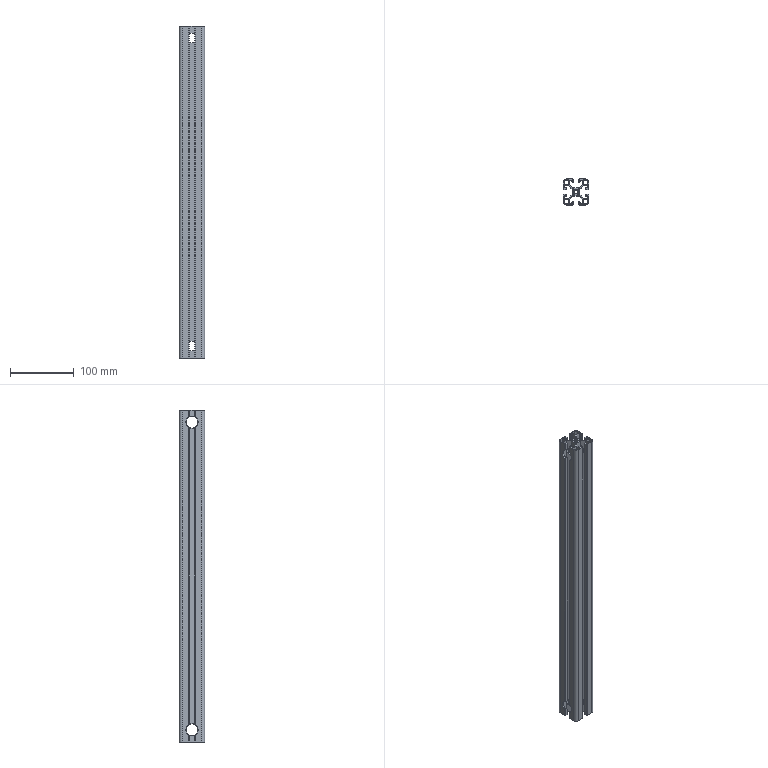Part | SolidWorks | features BaseBody 1, HoleWzd 1, MoveFace 1 | 1 solid | 235 faces | box 40 x 40 x 521 mm | volume 219782 mm3 | plane 166 | cylinder 69 | commonest cylinder face diameters 1.5 x18 2 x16 6.8 x15 19 x12 6.6 x4 9 x4